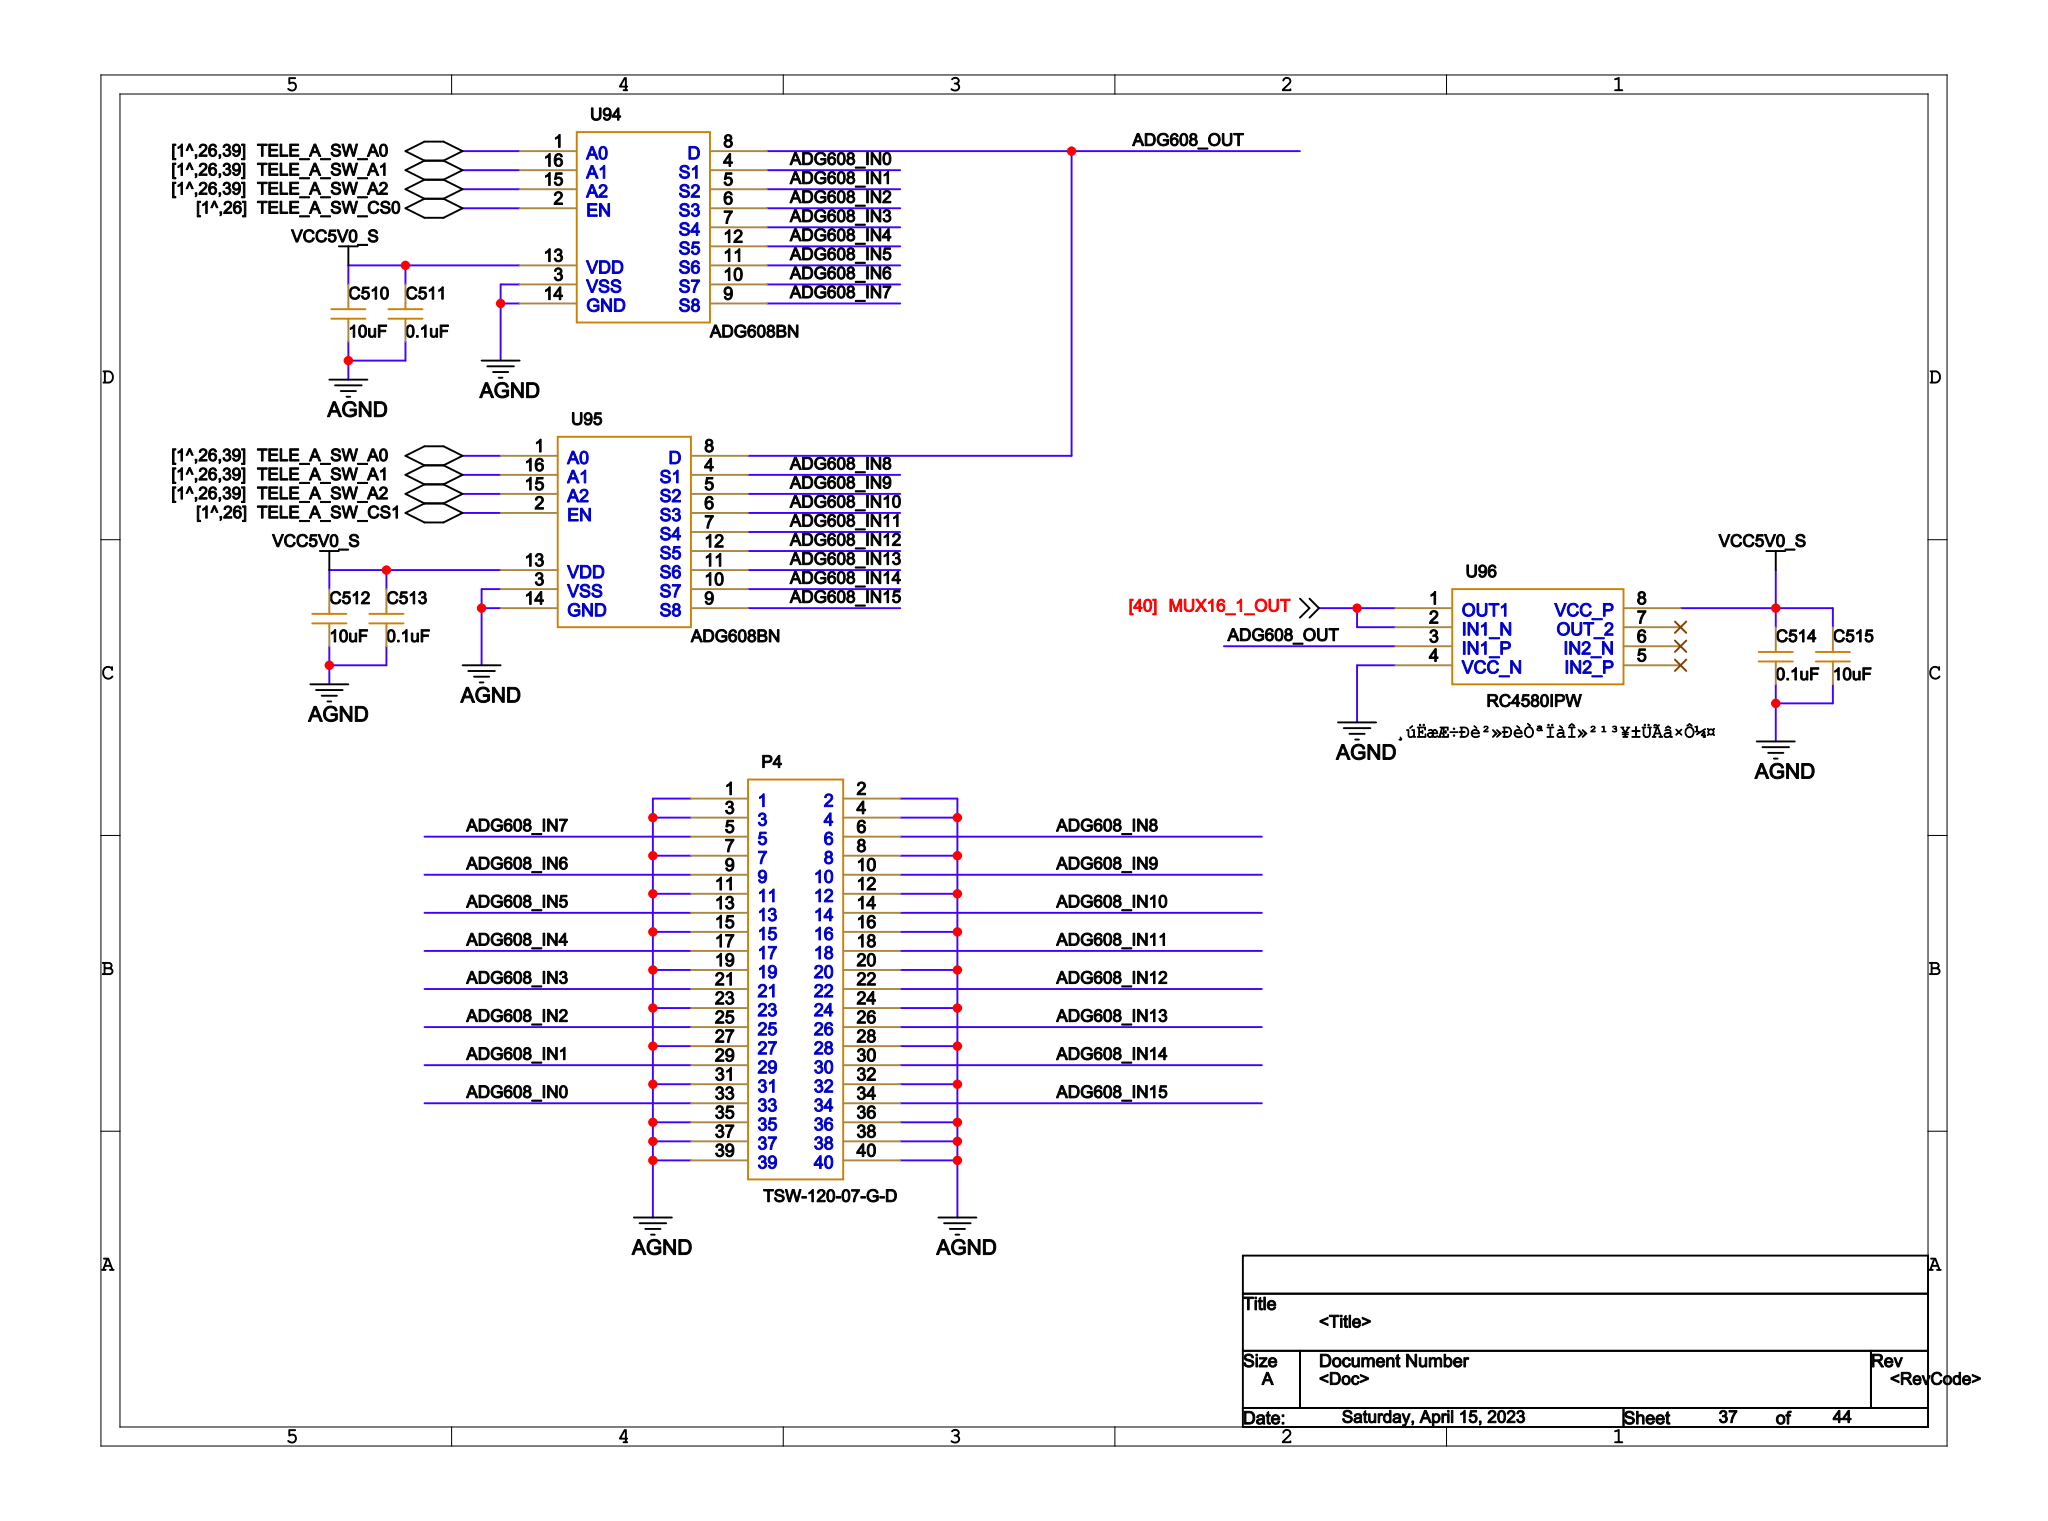Circuit board | Cadence Allegro | 1034 parts | 912 nets | one sheet of the schematic
Parts on this sheet (reference | value | footprint):
C510 | 10uF | C0402
C511 | 0.1uF | C0402
C512 | 10uF | C0402
C513 | 0.1uF | C0402
C514 | 0.1uF | C0402
C515 | 10uF | C0402
P4 | TSW-120-07-G-D | TSW_2MM54_DR
U94 | ADG608BN | ADG608_FP16
U95 | ADG608BN | ADG608_FP16
U96 | RC4580IPW | RC4580_TSSOP8
Nets of these parts (net: part-pin ...):
N234863: U94-1 U95-1
N234865: U94-16 U95-16
N234867: U94-15 U95-15
ADG608_OUT: U94-8 U95-8 U96-3
N234869: U94-2
AGND: C510-1 C511-1 C512-1 C513-1 C514-1 C515-1 U94-3 U94-14 U95-3 U95-14 U96-4 P4-1 P4-2 P4-3 P4-4 P4-7 P4-8 P4-11 P4-12 P4-15 P4-16 P4-19 P4-20 P4-23 P4-24 P4-27 P4-28 P4-31 P4-32 P4-35 P4-36 P4-37 P4-38 P4-39 P4-40
ADG608_IN0: U94-4 P4-33
ADG608_IN1: U94-5 P4-29
ADG608_IN2: U94-6 P4-25
ADG608_IN3: U94-7 P4-21
ADG608_IN4: U94-12 P4-17
ADG608_IN5: U94-11 P4-13
ADG608_IN6: U94-10 P4-9
ADG608_IN7: U94-9 P4-5
VCC5V0_S: C510-2 C511-2 C512-2 C513-2 C514-2 C515-2 U94-13 U95-13 U96-8
N234871: U95-2
ADG608_IN8: U95-4 P4-6
ADG608_IN9: U95-5 P4-10
ADG608_IN10: U95-6 P4-14
ADG608_IN11: U95-7 P4-18
ADG608_IN12: U95-12 P4-22
ADG608_IN13: U95-11 P4-26
ADG608_IN14: U95-10 P4-30
ADG608_IN15: U95-9 P4-34
MUX16_1_OUT: U96-1 U96-2